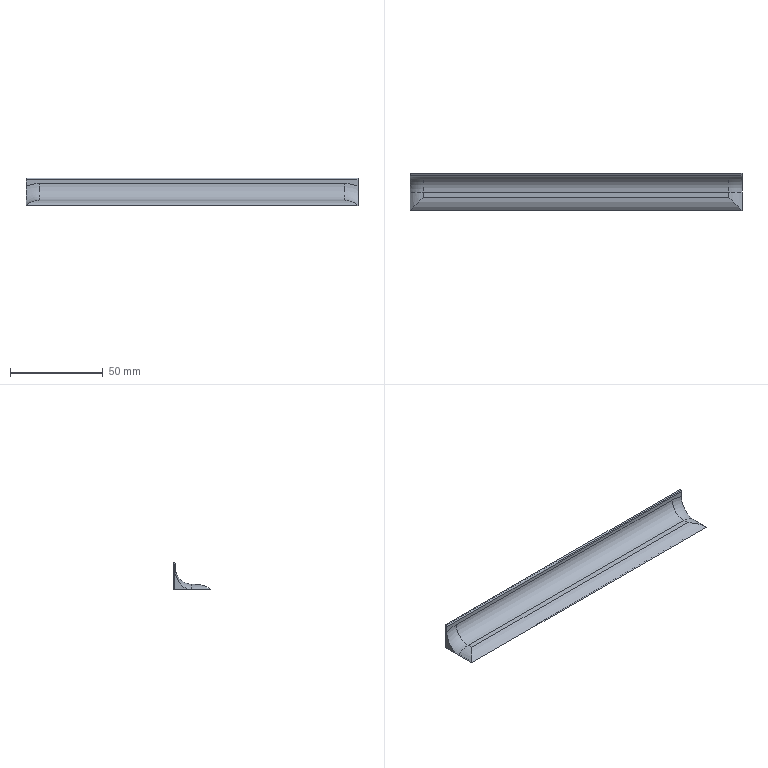Part | SolidWorks | features Fillet 3, ICE 2, Extrusion 1, Shell 1 | 1 solid | 23 faces | box 178.57 x 20 x 15 mm | volume 6954 mm3 | plane 12 | cylinder 9 | torus 2 | commonest cylinder face diameters 19 x4 20 x3 2 x1 18 x1
STEP:
#1=CARTESIAN_POINT('',(-88.785,9.5,0.));
#2=VERTEX_POINT('',#1);
#3=CARTESIAN_POINT('',(-88.785,10.,0.));
#4=VERTEX_POINT('',#3);
#5=CARTESIAN_POINT('',(-88.785,9.5,0.));
#6=DIRECTION('',(0.,1.,0.));
#7=VECTOR('',#6,1000.);
#8=LINE('',#5,#7);
#9=EDGE_CURVE('',#2,#4,#8,.T.);
#10=ORIENTED_EDGE('',*,*,#9,.F.);
#11=CARTESIAN_POINT('',(88.785,9.5,0.));
#12=VERTEX_POINT('',#11);
#13=CARTESIAN_POINT('',(-88.785,9.5,0.));
#14=DIRECTION('',(-1.,0.,0.));
#15=VECTOR('',#14,1000.);
#16=LINE('',#13,#15);
#17=EDGE_CURVE('',#12,#2,#16,.T.);
#18=ORIENTED_EDGE('',*,*,#17,.F.);
#19=CARTESIAN_POINT('',(88.785,10.,0.));
#20=VERTEX_POINT('',#19);
#21=CARTESIAN_POINT('',(88.785,9.5,0.));
#22=DIRECTION('',(0.,1.,0.));
#23=VECTOR('',#22,1000.);
#24=LINE('',#21,#23);
#25=EDGE_CURVE('',#12,#20,#24,.T.);
#26=ORIENTED_EDGE('',*,*,#25,.T.);
#27=CARTESIAN_POINT('',(89.285,10.,0.));
#28=VERTEX_POINT('',#27);
#29=CARTESIAN_POINT('',(-89.285,10.,0.));
#30=DIRECTION('',(-1.,0.,0.));
#31=VECTOR('',#30,1000.);
#32=LINE('',#29,#31);
#33=EDGE_CURVE('',#28,#20,#32,.T.);
#34=ORIENTED_EDGE('',*,*,#33,.F.);
#35=CARTESIAN_POINT('',(89.285,0.,0.));
#36=VERTEX_POINT('',#35);
#37=CARTESIAN_POINT('',(89.285,10.,0.));
#38=DIRECTION('',(0.,-1.,0.));
#39=VECTOR('',#38,1000.);
#40=LINE('',#37,#39);
#41=EDGE_CURVE('',#28,#36,#40,.T.);
#42=ORIENTED_EDGE('',*,*,#41,.T.);
#43=CARTESIAN_POINT('',(89.285,-10.,0.));
#44=VERTEX_POINT('',#43);
#45=CARTESIAN_POINT('',(89.285,-10.,0.));
#46=DIRECTION('',(0.,1.,0.));
#47=VECTOR('',#46,1000.);
#48=LINE('',#45,#47);
#49=EDGE_CURVE('',#44,#36,#48,.T.);
#50=ORIENTED_EDGE('',*,*,#49,.F.);
#51=CARTESIAN_POINT('',(-89.285,-10.,0.));
#52=VERTEX_POINT('',#51);
#53=CARTESIAN_POINT('',(-89.285,-10.,0.));
#54=DIRECTION('',(1.,0.,0.));
#55=VECTOR('',#54,1000.);
#56=LINE('',#53,#55);
#57=EDGE_CURVE('',#52,#44,#56,.T.);
#58=ORIENTED_EDGE('',*,*,#57,.F.);
#59=CARTESIAN_POINT('',(-89.285,0.,0.));
#60=VERTEX_POINT('',#59);
#61=CARTESIAN_POINT('',(-89.285,-10.,0.));
#62=DIRECTION('',(0.,-1.,0.));
#63=VECTOR('',#62,1000.);
#64=LINE('',#61,#63);
#65=EDGE_CURVE('',#60,#52,#64,.T.);
#66=ORIENTED_EDGE('',*,*,#65,.F.);
#67=CARTESIAN_POINT('',(-89.285,10.,0.));
#68=VERTEX_POINT('',#67);
#69=CARTESIAN_POINT('',(-89.285,-10.,0.));
#70=DIRECTION('',(0.,-1.,0.));
#71=VECTOR('',#70,1000.);
#72=LINE('',#69,#71);
#73=EDGE_CURVE('',#68,#60,#72,.T.);
#74=ORIENTED_EDGE('',*,*,#73,.F.);
#75=CARTESIAN_POINT('',(-89.285,10.,0.));
#76=DIRECTION('',(-1.,0.,0.));
#77=VECTOR('',#76,1000.);
#78=LINE('',#75,#77);
#79=EDGE_CURVE('',#4,#68,#78,.T.);
#80=ORIENTED_EDGE('',*,*,#79,.F.);
#81=EDGE_LOOP('',(#10,#18,#26,#34,#42,#50,#58,#66,#74,#80));
#82=FACE_OUTER_BOUND('',#81,.T.);
#83=CARTESIAN_POINT('',(88.566,-9.281,0.));
#84=VERTEX_POINT('',#83);
#85=CARTESIAN_POINT('',(88.566,9.,0.));
#86=VERTEX_POINT('',#85);
#87=CARTESIAN_POINT('',(88.566,-9.281,0.));
#88=DIRECTION('',(0.,1.,0.));
#89=VECTOR('',#88,1000.);
#90=LINE('',#87,#89);
#91=EDGE_CURVE('',#84,#86,#90,.T.);
#92=ORIENTED_EDGE('',*,*,#91,.T.);
#93=CARTESIAN_POINT('',(-88.566,9.,0.));
#94=VERTEX_POINT('',#93);
#95=CARTESIAN_POINT('',(89.285,9.,0.));
#96=DIRECTION('',(-1.,0.,0.));
#97=VECTOR('',#96,1000.);
#98=LINE('',#95,#97);
#99=EDGE_CURVE('',#86,#94,#98,.T.);
#100=ORIENTED_EDGE('',*,*,#99,.T.);
#101=CARTESIAN_POINT('',(-88.566,-9.281,0.));
#102=VERTEX_POINT('',#101);
#103=CARTESIAN_POINT('',(-88.566,9.281,0.));
#104=DIRECTION('',(0.,-1.,0.));
#105=VECTOR('',#104,1000.);
#106=LINE('',#103,#105);
#107=EDGE_CURVE('',#94,#102,#106,.T.);
#108=ORIENTED_EDGE('',*,*,#107,.T.);
#109=CARTESIAN_POINT('',(-88.566,-9.281,0.));
#110=DIRECTION('',(1.,0.,0.));
#111=VECTOR('',#110,1000.);
#112=LINE('',#109,#111);
#113=EDGE_CURVE('',#102,#84,#112,.T.);
#114=ORIENTED_EDGE('',*,*,#113,.T.);
#115=EDGE_LOOP('',(#92,#100,#108,#114));
#116=FACE_BOUND('',#115,.T.);
#117=CARTESIAN_POINT('',(0.,0.,0.));
#118=DIRECTION('',(0.,0.,-1.));
#119=DIRECTION('',(-1.,0.,0.));
#120=AXIS2_PLACEMENT_3D('',#117,#118,#119);
#121=PLANE('',#120);
#122=ADVANCED_FACE('',(#82,#116),#121,.T.);
#123=CARTESIAN_POINT('',(82.144,-2.859,3.));
#124=VERTEX_POINT('',#123);
#125=CARTESIAN_POINT('',(82.144,0.,3.));
#126=VERTEX_POINT('',#125);
#127=CARTESIAN_POINT('',(82.144,0.,3.));
#128=DIRECTION('',(0.,1.,0.));
#129=VECTOR('',#128,1000.);
#130=LINE('',#127,#129);
#131=EDGE_CURVE('',#124,#126,#130,.T.);
#132=ORIENTED_EDGE('',*,*,#131,.T.);
#133=CARTESIAN_POINT('',(-82.144,0.,3.));
#134=VERTEX_POINT('',#133);
#135=CARTESIAN_POINT('',(0.,0.,3.));
#136=DIRECTION('',(-1.,0.,0.));
#137=VECTOR('',#136,1000.);
#138=LINE('',#135,#137);
#139=EDGE_CURVE('',#126,#134,#138,.T.);
#140=ORIENTED_EDGE('',*,*,#139,.T.);
#141=CARTESIAN_POINT('',(-82.144,-2.859,3.));
#142=VERTEX_POINT('',#141);
#143=CARTESIAN_POINT('',(-82.144,0.,3.));
#144=DIRECTION('',(0.,-1.,0.));
#145=VECTOR('',#144,1000.);
#146=LINE('',#143,#145);
#147=EDGE_CURVE('',#134,#142,#146,.T.);
#148=ORIENTED_EDGE('',*,*,#147,.T.);
#149=CARTESIAN_POINT('',(0.,-2.859,3.));
#150=DIRECTION('',(1.,0.,0.));
#151=VECTOR('',#150,1000.);
#152=LINE('',#149,#151);
#153=EDGE_CURVE('',#142,#124,#152,.T.);
#154=ORIENTED_EDGE('',*,*,#153,.T.);
#155=EDGE_LOOP('',(#132,#140,#148,#154));
#156=FACE_OUTER_BOUND('',#155,.T.);
#157=CARTESIAN_POINT('',(0.,0.,3.));
#158=DIRECTION('',(0.,0.,-1.));
#159=DIRECTION('',(-1.,0.,0.));
#160=AXIS2_PLACEMENT_3D('',#157,#158,#159);
#161=PLANE('',#160);
#162=ADVANCED_FACE('',(#156),#161,.F.);
#163=ORIENTED_EDGE('',*,*,#147,.F.);
#164=CARTESIAN_POINT('',(-82.144,0.,-7.));
#165=DIRECTION('',(0.,-1.,0.));
#166=DIRECTION('',(0.,0.,-1.));
#167=AXIS2_PLACEMENT_3D('',#164,#165,#166);
#168=CIRCLE('',#167,10.);
#169=EDGE_CURVE('',#134,#60,#168,.T.);
#170=ORIENTED_EDGE('',*,*,#169,.T.);
#171=ORIENTED_EDGE('',*,*,#65,.T.);
#172=CARTESIAN_POINT('',(-82.144,-2.859,3.));
#173=CARTESIAN_POINT('',(-84.867,-5.582,3.));
#174=CARTESIAN_POINT('',(-87.378,-8.093,1.945));
#175=CARTESIAN_POINT('',(-89.285,-10.,0.));
#176=(BOUNDED_CURVE()B_SPLINE_CURVE(3,(#172,#173,#174,#175),.UNSPECIFIED.,.F.,.F.)B_SPLINE_CURVE_WITH_KNOTS((4,4),(1.571,2.366),.UNSPECIFIED.)CURVE()GEOMETRIC_REPRESENTATION_ITEM()RATIONAL_B_SPLINE_CURVE((1.,0.948,0.948,1.))REPRESENTATION_ITEM(''));
#177=EDGE_CURVE('',#142,#52,#176,.T.);
#178=ORIENTED_EDGE('',*,*,#177,.F.);
#179=EDGE_LOOP('',(#163,#170,#171,#178));
#180=FACE_OUTER_BOUND('',#179,.T.);
#181=CARTESIAN_POINT('',(-82.144,-10.,-7.));
#182=DIRECTION('',(0.,1.,0.));
#183=DIRECTION('',(0.,0.,1.));
#184=AXIS2_PLACEMENT_3D('',#181,#182,#183);
#185=CYLINDRICAL_SURFACE('',#184,10.);
#186=ADVANCED_FACE('',(#180),#185,.T.);
#187=ORIENTED_EDGE('',*,*,#49,.T.);
#188=CARTESIAN_POINT('',(82.144,0.,-7.));
#189=DIRECTION('',(0.,-1.,0.));
#190=DIRECTION('',(0.,0.,-1.));
#191=AXIS2_PLACEMENT_3D('',#188,#189,#190);
#192=CIRCLE('',#191,10.);
#193=EDGE_CURVE('',#36,#126,#192,.T.);
#194=ORIENTED_EDGE('',*,*,#193,.T.);
#195=ORIENTED_EDGE('',*,*,#131,.F.);
#196=CARTESIAN_POINT('',(89.285,-10.,0.));
#197=CARTESIAN_POINT('',(87.378,-8.093,1.945));
#198=CARTESIAN_POINT('',(84.867,-5.582,3.));
#199=CARTESIAN_POINT('',(82.144,-2.859,3.));
#200=(BOUNDED_CURVE()B_SPLINE_CURVE(3,(#196,#197,#198,#199),.UNSPECIFIED.,.F.,.F.)B_SPLINE_CURVE_WITH_KNOTS((4,4),(0.7754,1.571),.UNSPECIFIED.)CURVE()GEOMETRIC_REPRESENTATION_ITEM()RATIONAL_B_SPLINE_CURVE((1.,0.948,0.948,1.))REPRESENTATION_ITEM(''));
#201=EDGE_CURVE('',#44,#124,#200,.T.);
#202=ORIENTED_EDGE('',*,*,#201,.F.);
#203=EDGE_LOOP('',(#187,#194,#195,#202));
#204=FACE_OUTER_BOUND('',#203,.T.);
#205=CARTESIAN_POINT('',(82.144,-10.,-7.));
#206=DIRECTION('',(0.,-1.,0.));
#207=DIRECTION('',(0.,0.,-1.));
#208=AXIS2_PLACEMENT_3D('',#205,#206,#207);
#209=CYLINDRICAL_SURFACE('',#208,10.);
#210=ADVANCED_FACE('',(#204),#209,.T.);
#211=ORIENTED_EDGE('',*,*,#177,.T.);
#212=ORIENTED_EDGE('',*,*,#57,.T.);
#213=ORIENTED_EDGE('',*,*,#201,.T.);
#214=ORIENTED_EDGE('',*,*,#153,.F.);
#215=EDGE_LOOP('',(#211,#212,#213,#214));
#216=FACE_OUTER_BOUND('',#215,.T.);
#217=CARTESIAN_POINT('',(-89.285,-2.859,-7.));
#218=DIRECTION('',(-1.,0.,0.));
#219=DIRECTION('',(0.,0.,1.));
#220=AXIS2_PLACEMENT_3D('',#217,#218,#219);
#221=CYLINDRICAL_SURFACE('',#220,10.);
#222=ADVANCED_FACE('',(#216),#221,.T.);
#223=CARTESIAN_POINT('',(-82.144,2.859,2.5));
#224=VERTEX_POINT('',#223);
#225=CARTESIAN_POINT('',(-82.144,-2.859,2.5));
#226=VERTEX_POINT('',#225);
#227=CARTESIAN_POINT('',(-82.144,0.,2.5));
#228=DIRECTION('',(0.,-1.,0.));
#229=VECTOR('',#228,1000.);
#230=LINE('',#227,#229);
#231=EDGE_CURVE('',#224,#226,#230,.T.);
#232=ORIENTED_EDGE('',*,*,#231,.F.);
#233=CARTESIAN_POINT('',(82.144,2.859,2.5));
#234=VERTEX_POINT('',#233);
#235=CARTESIAN_POINT('',(0.,2.859,2.5));
#236=DIRECTION('',(-1.,0.,0.));
#237=VECTOR('',#236,1000.);
#238=LINE('',#235,#237);
#239=EDGE_CURVE('',#234,#224,#238,.T.);
#240=ORIENTED_EDGE('',*,*,#239,.F.);
#241=CARTESIAN_POINT('',(82.144,-2.859,2.5));
#242=VERTEX_POINT('',#241);
#243=CARTESIAN_POINT('',(82.144,0.,2.5));
#244=DIRECTION('',(0.,1.,0.));
#245=VECTOR('',#244,1000.);
#246=LINE('',#243,#245);
#247=EDGE_CURVE('',#242,#234,#246,.T.);
#248=ORIENTED_EDGE('',*,*,#247,.F.);
#249=CARTESIAN_POINT('',(0.,-2.859,2.5));
#250=DIRECTION('',(1.,0.,0.));
#251=VECTOR('',#250,1000.);
#252=LINE('',#249,#251);
#253=EDGE_CURVE('',#226,#242,#252,.T.);
#254=ORIENTED_EDGE('',*,*,#253,.F.);
#255=EDGE_LOOP('',(#232,#240,#248,#254));
#256=FACE_OUTER_BOUND('',#255,.T.);
#257=CARTESIAN_POINT('',(0.,0.,2.5));
#258=DIRECTION('',(0.,0.,-1.));
#259=DIRECTION('',(-1.,0.,0.));
#260=AXIS2_PLACEMENT_3D('',#257,#258,#259);
#261=PLANE('',#260);
#262=ADVANCED_FACE('',(#256),#261,.T.);
#263=CARTESIAN_POINT('',(-88.285,9.,0.248));
#264=VERTEX_POINT('',#263);
#265=CARTESIAN_POINT('',(-82.144,2.859,2.5));
#266=CARTESIAN_POINT('',(-84.417,5.132,2.5));
#267=CARTESIAN_POINT('',(-86.551,7.266,1.717));
#268=CARTESIAN_POINT('',(-88.285,9.,0.248));
#269=(BOUNDED_CURVE()B_SPLINE_CURVE(3,(#265,#266,#267,#268),.UNSPECIFIED.,.F.,.F.)B_SPLINE_CURVE_WITH_KNOTS((4,4),(4.712,5.415),.UNSPECIFIED.)CURVE()GEOMETRIC_REPRESENTATION_ITEM()RATIONAL_B_SPLINE_CURVE((1.,0.9592,0.9592,1.))REPRESENTATION_ITEM(''));
#270=EDGE_CURVE('',#224,#264,#269,.T.);
#271=ORIENTED_EDGE('',*,*,#270,.T.);
#272=CARTESIAN_POINT('',(88.285,9.,0.248));
#273=VERTEX_POINT('',#272);
#274=CARTESIAN_POINT('',(-89.285,9.,0.248));
#275=DIRECTION('',(1.,0.,0.));
#276=VECTOR('',#275,1000.);
#277=LINE('',#274,#276);
#278=EDGE_CURVE('',#264,#273,#277,.T.);
#279=ORIENTED_EDGE('',*,*,#278,.T.);
#280=CARTESIAN_POINT('',(88.285,9.,0.248));
#281=CARTESIAN_POINT('',(86.551,7.266,1.717));
#282=CARTESIAN_POINT('',(84.417,5.132,2.5));
#283=CARTESIAN_POINT('',(82.144,2.859,2.5));
#284=(BOUNDED_CURVE()B_SPLINE_CURVE(3,(#280,#281,#282,#283),.UNSPECIFIED.,.F.,.F.)B_SPLINE_CURVE_WITH_KNOTS((4,4),(4.009,4.712),.UNSPECIFIED.)CURVE()GEOMETRIC_REPRESENTATION_ITEM()RATIONAL_B_SPLINE_CURVE((1.,0.9592,0.9592,1.))REPRESENTATION_ITEM(''));
#285=EDGE_CURVE('',#273,#234,#284,.T.);
#286=ORIENTED_EDGE('',*,*,#285,.T.);
#287=ORIENTED_EDGE('',*,*,#239,.T.);
#288=EDGE_LOOP('',(#271,#279,#286,#287));
#289=FACE_OUTER_BOUND('',#288,.T.);
#290=CARTESIAN_POINT('',(-89.285,2.859,-7.));
#291=DIRECTION('',(1.,0.,0.));
#292=DIRECTION('',(0.,0.,-1.));
#293=AXIS2_PLACEMENT_3D('',#290,#291,#292);
#294=CYLINDRICAL_SURFACE('',#293,9.5);
#295=ADVANCED_FACE('',(#289),#294,.F.);
#296=ORIENTED_EDGE('',*,*,#107,.F.);
#297=CARTESIAN_POINT('',(-82.144,9.,-7.));
#298=DIRECTION('',(0.,1.,0.));
#299=DIRECTION('',(0.,0.,-1.));
#300=AXIS2_PLACEMENT_3D('',#297,#298,#299);
#301=CIRCLE('',#300,9.5);
#302=EDGE_CURVE('',#94,#264,#301,.T.);
#303=ORIENTED_EDGE('',*,*,#302,.T.);
#304=ORIENTED_EDGE('',*,*,#270,.F.);
#305=ORIENTED_EDGE('',*,*,#231,.T.);
#306=CARTESIAN_POINT('',(-82.144,-2.859,2.5));
#307=CARTESIAN_POINT('',(-84.55,-5.265,2.5));
#308=CARTESIAN_POINT('',(-86.793,-7.508,1.627));
#309=CARTESIAN_POINT('',(-88.566,-9.281,0.));
#310=(BOUNDED_CURVE()B_SPLINE_CURVE(3,(#306,#307,#308,#309),.UNSPECIFIED.,.F.,.F.)B_SPLINE_CURVE_WITH_KNOTS((4,4),(4.712,5.455),.UNSPECIFIED.)CURVE()GEOMETRIC_REPRESENTATION_ITEM()RATIONAL_B_SPLINE_CURVE((1.,0.9546,0.9546,1.))REPRESENTATION_ITEM(''));
#311=EDGE_CURVE('',#226,#102,#310,.T.);
#312=ORIENTED_EDGE('',*,*,#311,.T.);
#313=EDGE_LOOP('',(#296,#303,#304,#305,#312));
#314=FACE_OUTER_BOUND('',#313,.T.);
#315=CARTESIAN_POINT('',(-82.144,-10.,-7.));
#316=DIRECTION('',(0.,1.,0.));
#317=DIRECTION('',(0.,0.,1.));
#318=AXIS2_PLACEMENT_3D('',#315,#316,#317);
#319=CYLINDRICAL_SURFACE('',#318,9.5);
#320=ADVANCED_FACE('',(#314),#319,.F.);
#321=ORIENTED_EDGE('',*,*,#285,.F.);
#322=CARTESIAN_POINT('',(82.144,9.,-7.));
#323=DIRECTION('',(0.,1.,0.));
#324=DIRECTION('',(0.,0.,-1.));
#325=AXIS2_PLACEMENT_3D('',#322,#323,#324);
#326=CIRCLE('',#325,9.5);
#327=EDGE_CURVE('',#273,#86,#326,.T.);
#328=ORIENTED_EDGE('',*,*,#327,.T.);
#329=ORIENTED_EDGE('',*,*,#91,.F.);
#330=CARTESIAN_POINT('',(88.566,-9.281,0.));
#331=CARTESIAN_POINT('',(86.793,-7.508,1.627));
#332=CARTESIAN_POINT('',(84.55,-5.265,2.5));
#333=CARTESIAN_POINT('',(82.144,-2.859,2.5));
#334=(BOUNDED_CURVE()B_SPLINE_CURVE(3,(#330,#331,#332,#333),.UNSPECIFIED.,.F.,.F.)B_SPLINE_CURVE_WITH_KNOTS((4,4),(3.97,4.712),.UNSPECIFIED.)CURVE()GEOMETRIC_REPRESENTATION_ITEM()RATIONAL_B_SPLINE_CURVE((1.,0.9546,0.9546,1.))REPRESENTATION_ITEM(''));
#335=EDGE_CURVE('',#84,#242,#334,.T.);
#336=ORIENTED_EDGE('',*,*,#335,.T.);
#337=ORIENTED_EDGE('',*,*,#247,.T.);
#338=EDGE_LOOP('',(#321,#328,#329,#336,#337));
#339=FACE_OUTER_BOUND('',#338,.T.);
#340=CARTESIAN_POINT('',(82.144,-10.,-7.));
#341=DIRECTION('',(0.,-1.,0.));
#342=DIRECTION('',(0.,0.,-1.));
#343=AXIS2_PLACEMENT_3D('',#340,#341,#342);
#344=CYLINDRICAL_SURFACE('',#343,9.5);
#345=ADVANCED_FACE('',(#339),#344,.F.);
#346=ORIENTED_EDGE('',*,*,#311,.F.);
#347=ORIENTED_EDGE('',*,*,#253,.T.);
#348=ORIENTED_EDGE('',*,*,#335,.F.);
#349=ORIENTED_EDGE('',*,*,#113,.F.);
#350=EDGE_LOOP('',(#346,#347,#348,#349));
#351=FACE_OUTER_BOUND('',#350,.T.);
#352=CARTESIAN_POINT('',(-89.285,-2.859,-7.));
#353=DIRECTION('',(-1.,0.,0.));
#354=DIRECTION('',(0.,0.,1.));
#355=AXIS2_PLACEMENT_3D('',#352,#353,#354);
#356=CYLINDRICAL_SURFACE('',#355,9.5);
#357=ADVANCED_FACE('',(#351),#356,.F.);
#358=ORIENTED_EDGE('',*,*,#302,.F.);
#359=ORIENTED_EDGE('',*,*,#99,.F.);
#360=ORIENTED_EDGE('',*,*,#327,.F.);
#361=ORIENTED_EDGE('',*,*,#278,.F.);
#362=EDGE_LOOP('',(#358,#359,#360,#361));
#363=FACE_OUTER_BOUND('',#362,.T.);
#364=CARTESIAN_POINT('',(89.285,9.,15.));
#365=DIRECTION('',(0.,-1.,0.));
#366=DIRECTION('',(0.,0.,-1.));
#367=AXIS2_PLACEMENT_3D('',#364,#365,#366);
#368=PLANE('',#367);
#369=ADVANCED_FACE('',(#363),#368,.T.);
#370=CARTESIAN_POINT('',(89.285,10.,15.));
#371=VERTEX_POINT('',#370);
#372=CARTESIAN_POINT('',(89.285,10.,15.));
#373=DIRECTION('',(0.,0.,-1.));
#374=VECTOR('',#373,1000.);
#375=LINE('',#372,#374);
#376=EDGE_CURVE('',#371,#28,#375,.T.);
#377=ORIENTED_EDGE('',*,*,#376,.F.);
#378=CARTESIAN_POINT('',(89.285,9.,14.));
#379=VERTEX_POINT('',#378);
#380=CARTESIAN_POINT('',(89.285,10.,14.));
#381=DIRECTION('',(1.,0.,0.));
#382=DIRECTION('',(0.,0.,-1.));
#383=AXIS2_PLACEMENT_3D('',#380,#381,#382);
#384=CIRCLE('',#383,1.);
#385=EDGE_CURVE('',#371,#379,#384,.T.);
#386=ORIENTED_EDGE('',*,*,#385,.T.);
#387=CARTESIAN_POINT('',(89.285,9.,10.607));
#388=VERTEX_POINT('',#387);
#389=CARTESIAN_POINT('',(89.285,9.,15.));
#390=DIRECTION('',(0.,0.,-1.));
#391=VECTOR('',#390,1000.);
#392=LINE('',#389,#391);
#393=EDGE_CURVE('',#379,#388,#392,.T.);
#394=ORIENTED_EDGE('',*,*,#393,.T.);
#395=CARTESIAN_POINT('',(89.285,9.,10.607));
#396=CARTESIAN_POINT('',(89.285,9.,9.965));
#397=CARTESIAN_POINT('',(89.285,8.942,9.334));
#398=CARTESIAN_POINT('',(89.285,8.718,8.09));
#399=CARTESIAN_POINT('',(89.285,8.553,7.476));
#400=CARTESIAN_POINT('',(89.285,8.117,6.272));
#401=CARTESIAN_POINT('',(89.285,7.851,5.696));
#402=CARTESIAN_POINT('',(89.285,7.387,4.868));
#403=CARTESIAN_POINT('',(89.285,7.221,4.599));
#404=CARTESIAN_POINT('',(89.285,6.866,4.072));
#405=CARTESIAN_POINT('',(89.285,6.676,3.813));
#406=CARTESIAN_POINT('',(89.285,6.078,3.064));
#407=CARTESIAN_POINT('',(89.285,5.644,2.604));
#408=CARTESIAN_POINT('',(89.285,4.701,1.766));
#409=CARTESIAN_POINT('',(89.285,4.193,1.387));
#410=CARTESIAN_POINT('',(89.285,3.087,0.7335));
#411=CARTESIAN_POINT('',(89.285,2.508,0.4703));
#412=CARTESIAN_POINT('',(89.285,1.591,0.1935));
#413=CARTESIAN_POINT('',(89.285,1.275,0.1212));
#414=CARTESIAN_POINT('',(89.285,0.6417,0.02471));
#415=CARTESIAN_POINT('',(89.285,0.3223,0.));
#416=CARTESIAN_POINT('',(89.285,0.,0.));
#417=B_SPLINE_CURVE_WITH_KNOTS('',3,(#395,#396,#397,#398,#399,#400,#401,#402,#403,#404,#405,#406,#407,#408,#409,#410,#411,#412,#413,#414,#415,#416),.UNSPECIFIED.,.F.,.F.,(4,2,2,2,2,2,2,2,2,2,4),(0.,0.001896,0.003792,0.005687,0.006635,0.007583,0.009479,0.01137,0.01327,0.01422,0.01517),.UNSPECIFIED.);
#418=EDGE_CURVE('',#388,#36,#417,.T.);
#419=ORIENTED_EDGE('',*,*,#418,.T.);
#420=ORIENTED_EDGE('',*,*,#41,.F.);
#421=EDGE_LOOP('',(#377,#386,#394,#419,#420));
#422=FACE_OUTER_BOUND('',#421,.T.);
#423=CARTESIAN_POINT('',(89.285,10.,15.));
#424=DIRECTION('',(1.,0.,0.));
#425=DIRECTION('',(0.,0.,-1.));
#426=AXIS2_PLACEMENT_3D('',#423,#424,#425);
#427=PLANE('',#426);
#428=ADVANCED_FACE('',(#422),#427,.T.);
#429=CARTESIAN_POINT('',(-88.785,10.,14.5));
#430=VERTEX_POINT('',#429);
#431=CARTESIAN_POINT('',(-88.785,10.,0.));
#432=DIRECTION('',(0.,0.,1.));
#433=VECTOR('',#432,1000.);
#434=LINE('',#431,#433);
#435=EDGE_CURVE('',#4,#430,#434,.T.);
#436=ORIENTED_EDGE('',*,*,#435,.F.);
#437=ORIENTED_EDGE('',*,*,#79,.T.);
#438=CARTESIAN_POINT('',(-89.285,10.,15.));
#439=VERTEX_POINT('',#438);
#440=CARTESIAN_POINT('',(-89.285,10.,15.));
#441=DIRECTION('',(0.,0.,-1.));
#442=VECTOR('',#441,1000.);
#443=LINE('',#440,#442);
#444=EDGE_CURVE('',#439,#68,#443,.T.);
#445=ORIENTED_EDGE('',*,*,#444,.F.);
#446=CARTESIAN_POINT('',(89.285,10.,15.));
#447=DIRECTION('',(1.,0.,0.));
#448=VECTOR('',#447,1000.);
#449=LINE('',#446,#448);
#450=EDGE_CURVE('',#439,#371,#449,.T.);
#451=ORIENTED_EDGE('',*,*,#450,.T.);
#452=ORIENTED_EDGE('',*,*,#376,.T.);
#453=ORIENTED_EDGE('',*,*,#33,.T.);
#454=CARTESIAN_POINT('',(88.785,10.,14.5));
#455=VERTEX_POINT('',#454);
#456=CARTESIAN_POINT('',(88.785,10.,0.));
#457=DIRECTION('',(0.,0.,-1.));
#458=VECTOR('',#457,1000.);
#459=LINE('',#456,#458);
#460=EDGE_CURVE('',#455,#20,#459,.T.);
#461=ORIENTED_EDGE('',*,*,#460,.F.);
#462=CARTESIAN_POINT('',(-88.785,10.,14.5));
#463=DIRECTION('',(1.,0.,0.));
#464=VECTOR('',#463,1000.);
#465=LINE('',#462,#464);
#466=EDGE_CURVE('',#430,#455,#465,.T.);
#467=ORIENTED_EDGE('',*,*,#466,.F.);
#468=EDGE_LOOP('',(#436,#437,#445,#451,#452,#453,#461,#467));
#469=FACE_OUTER_BOUND('',#468,.T.);
#470=CARTESIAN_POINT('',(89.285,10.,15.));
#471=DIRECTION('',(0.,1.,0.));
#472=DIRECTION('',(0.,0.,1.));
#473=AXIS2_PLACEMENT_3D('',#470,#471,#472);
#474=PLANE('',#473);
#475=ADVANCED_FACE('',(#469),#474,.T.);
#476=CARTESIAN_POINT('',(-89.285,9.,14.));
#477=VERTEX_POINT('',#476);
#478=CARTESIAN_POINT('',(-89.285,9.,10.607));
#479=VERTEX_POINT('',#478);
#480=CARTESIAN_POINT('',(-89.285,9.,15.));
#481=DIRECTION('',(0.,0.,-1.));
#482=VECTOR('',#481,1000.);
#483=LINE('',#480,#482);
#484=EDGE_CURVE('',#477,#479,#483,.T.);
#485=ORIENTED_EDGE('',*,*,#484,.F.);
#486=CARTESIAN_POINT('',(-89.285,10.,14.));
#487=DIRECTION('',(-1.,0.,0.));
#488=DIRECTION('',(0.,0.,1.));
#489=AXIS2_PLACEMENT_3D('',#486,#487,#488);
#490=CIRCLE('',#489,1.);
#491=EDGE_CURVE('',#477,#439,#490,.T.);
#492=ORIENTED_EDGE('',*,*,#491,.T.);
#493=ORIENTED_EDGE('',*,*,#444,.T.);
#494=ORIENTED_EDGE('',*,*,#73,.T.);
#495=CARTESIAN_POINT('',(-89.285,0.,0.));
#496=CARTESIAN_POINT('',(-89.285,0.6442,0.));
#497=CARTESIAN_POINT('',(-89.285,1.269,0.09828));
#498=CARTESIAN_POINT('',(-89.285,2.181,0.3709));
#499=CARTESIAN_POINT('',(-89.285,2.483,0.4837));
#500=CARTESIAN_POINT('',(-89.285,3.068,0.7434));
#501=CARTESIAN_POINT('',(-89.285,3.35,0.8899));
#502=CARTESIAN_POINT('',(-89.285,3.898,1.212));
#503=CARTESIAN_POINT('',(-89.285,4.163,1.388));
#504=CARTESIAN_POINT('',(-89.285,4.679,1.766));
#505=CARTESIAN_POINT('',(-89.285,4.928,1.968));
#506=CARTESIAN_POINT('',(-89.285,5.641,2.601));
#507=CARTESIAN_POINT('',(-89.285,6.075,3.061));
#508=CARTESIAN_POINT('',(-89.285,6.669,3.803));
#509=CARTESIAN_POINT('',(-89.285,6.857,4.059));
#510=CARTESIAN_POINT('',(-89.285,7.214,4.588));
#511=CARTESIAN_POINT('',(-89.285,7.382,4.861));
#512=CARTESIAN_POINT('',(-89.285,7.849,5.692));
#513=CARTESIAN_POINT('',(-89.285,8.114,6.266));
#514=CARTESIAN_POINT('',(-89.285,8.547,7.457));
#515=CARTESIAN_POINT('',(-89.285,8.716,8.078));
#516=CARTESIAN_POINT('',(-89.285,8.942,9.332));
#517=CARTESIAN_POINT('',(-89.285,9.,9.966));
#518=CARTESIAN_POINT('',(-89.285,9.,10.607));
#519=B_SPLINE_CURVE_WITH_KNOTS('',3,(#495,#496,#497,#498,#499,#500,#501,#502,#503,#504,#505,#506,#507,#508,#509,#510,#511,#512,#513,#514,#515,#516,#517,#518),.UNSPECIFIED.,.F.,.F.,(4,2,2,2,2,2,2,2,2,2,2,4),(0.,0.001896,0.002844,0.003792,0.00474,0.005688,0.007584,0.008532,0.00948,0.01138,0.01327,0.01517),.UNSPECIFIED.);
#520=EDGE_CURVE('',#60,#479,#519,.T.);
#521=ORIENTED_EDGE('',*,*,#520,.T.);
#522=EDGE_LOOP('',(#485,#492,#493,#494,#521));
#523=FACE_OUTER_BOUND('',#522,.T.);
#524=CARTESIAN_POINT('',(-89.285,10.,15.));
#525=DIRECTION('',(-1.,0.,0.));
#526=DIRECTION('',(0.,0.,1.));
#527=AXIS2_PLACEMENT_3D('',#524,#525,#526);
#528=PLANE('',#527);
#529=ADVANCED_FACE('',(#523),#528,.T.);
#530=ORIENTED_EDGE('',*,*,#393,.F.);
#531=CARTESIAN_POINT('',(-89.285,9.,14.));
#532=DIRECTION('',(-1.,0.,0.));
#533=VECTOR('',#532,1000.);
#534=LINE('',#531,#533);
#535=EDGE_CURVE('',#379,#477,#534,.T.);
#536=ORIENTED_EDGE('',*,*,#535,.T.);
#537=ORIENTED_EDGE('',*,*,#484,.T.);
#538=CARTESIAN_POINT('',(-82.144,9.,12.));
#539=VERTEX_POINT('',#538);
#540=CARTESIAN_POINT('',(-82.144,9.,-7.));
#541=DIRECTION('',(0.,1.,0.));
#542=DIRECTION('',(0.,0.,-1.));
#543=AXIS2_PLACEMENT_3D('',#540,#541,#542);
#544=CIRCLE('',#543,19.);
#545=EDGE_CURVE('',#479,#539,#544,.T.);
#546=ORIENTED_EDGE('',*,*,#545,.T.);
#547=CARTESIAN_POINT('',(82.144,9.,12.));
#548=VERTEX_POINT('',#547);
#549=CARTESIAN_POINT('',(89.285,9.,12.));
#550=DIRECTION('',(1.,0.,0.));
#551=VECTOR('',#550,1000.);
#552=LINE('',#549,#551);
#553=EDGE_CURVE('',#539,#548,#552,.T.);
#554=ORIENTED_EDGE('',*,*,#553,.T.);
#555=CARTESIAN_POINT('',(82.144,9.,-7.));
#556=DIRECTION('',(0.,1.,0.));
#557=DIRECTION('',(0.,0.,-1.));
#558=AXIS2_PLACEMENT_3D('',#555,#556,#557);
#559=CIRCLE('',#558,19.);
#560=EDGE_CURVE('',#548,#388,#559,.T.);
#561=ORIENTED_EDGE('',*,*,#560,.T.);
#562=EDGE_LOOP('',(#530,#536,#537,#546,#554,#561));
#563=FACE_OUTER_BOUND('',#562,.T.);
#564=CARTESIAN_POINT('',(89.285,9.,15.));
#565=DIRECTION('',(0.,-1.,0.));
#566=DIRECTION('',(0.,0.,-1.));
#567=AXIS2_PLACEMENT_3D('',#564,#565,#566);
#568=PLANE('',#567);
#569=ADVANCED_FACE('',(#563),#568,.T.);
#570=ORIENTED_EDGE('',*,*,#520,.F.);
#571=ORIENTED_EDGE('',*,*,#169,.F.);
#572=CARTESIAN_POINT('',(-82.144,0.,12.));
#573=DIRECTION('',(-1.,0.,0.));
#574=DIRECTION('',(0.,0.,-1.));
#575=AXIS2_PLACEMENT_3D('',#572,#573,#574);
#576=CIRCLE('',#575,9.);
#577=EDGE_CURVE('',#539,#134,#576,.T.);
#578=ORIENTED_EDGE('',*,*,#577,.F.);
#579=ORIENTED_EDGE('',*,*,#545,.F.);
#580=EDGE_LOOP('',(#570,#571,#578,#579));
#581=FACE_OUTER_BOUND('',#580,.T.);
#582=CARTESIAN_POINT('',(-82.144,0.,-7.));
#583=DIRECTION('',(0.,-1.,0.));
#584=DIRECTION('',(0.,0.,-1.));
#585=AXIS2_PLACEMENT_3D('',#582,#583,#584);
#586=TOROIDAL_SURFACE('',#585,19.,9.);
#587=ADVANCED_FACE('',(#581),#586,.F.);
#588=ORIENTED_EDGE('',*,*,#577,.T.);
#589=ORIENTED_EDGE('',*,*,#139,.F.);
#590=CARTESIAN_POINT('',(82.144,0.,12.));
#591=DIRECTION('',(-1.,0.,0.));
#592=DIRECTION('',(0.,0.,-1.));
#593=AXIS2_PLACEMENT_3D('',#590,#591,#592);
#594=CIRCLE('',#593,9.);
#595=EDGE_CURVE('',#548,#126,#594,.T.);
#596=ORIENTED_EDGE('',*,*,#595,.F.);
#597=ORIENTED_EDGE('',*,*,#553,.F.);
#598=EDGE_LOOP('',(#588,#589,#596,#597));
#599=FACE_OUTER_BOUND('',#598,.T.);
#600=CARTESIAN_POINT('',(89.285,0.,12.));
#601=DIRECTION('',(1.,0.,0.));
#602=DIRECTION('',(0.,0.,-1.));
#603=AXIS2_PLACEMENT_3D('',#600,#601,#602);
#604=CYLINDRICAL_SURFACE('',#603,9.);
#605=ADVANCED_FACE('',(#599),#604,.F.);
#606=ORIENTED_EDGE('',*,*,#595,.T.);
#607=ORIENTED_EDGE('',*,*,#193,.F.);
#608=ORIENTED_EDGE('',*,*,#418,.F.);
#609=ORIENTED_EDGE('',*,*,#560,.F.);
#610=EDGE_LOOP('',(#606,#607,#608,#609));
#611=FACE_OUTER_BOUND('',#610,.T.);
#612=CARTESIAN_POINT('',(82.144,0.,-7.));
#613=DIRECTION('',(0.,-1.,0.));
#614=DIRECTION('',(0.,0.,-1.));
#615=AXIS2_PLACEMENT_3D('',#612,#613,#614);
#616=TOROIDAL_SURFACE('',#615,19.,9.);
#617=ADVANCED_FACE('',(#611),#616,.F.);
#618=ORIENTED_EDGE('',*,*,#385,.F.);
#619=ORIENTED_EDGE('',*,*,#450,.F.);
#620=ORIENTED_EDGE('',*,*,#491,.F.);
#621=ORIENTED_EDGE('',*,*,#535,.F.);
#622=EDGE_LOOP('',(#618,#619,#620,#621));
#623=FACE_OUTER_BOUND('',#622,.T.);
#624=CARTESIAN_POINT('',(89.285,10.,14.));
#625=DIRECTION('',(1.,0.,0.));
#626=DIRECTION('',(0.,0.,-1.));
#627=AXIS2_PLACEMENT_3D('',#624,#625,#626);
#628=CYLINDRICAL_SURFACE('',#627,1.);
#629=ADVANCED_FACE('',(#623),#628,.T.);
#630=ORIENTED_EDGE('',*,*,#435,.T.);
#631=CARTESIAN_POINT('',(-88.785,9.5,14.5));
#632=VERTEX_POINT('',#631);
#633=CARTESIAN_POINT('',(-88.785,9.5,14.5));
#634=DIRECTION('',(0.,1.,0.));
#635=VECTOR('',#634,1000.);
#636=LINE('',#633,#635);
#637=EDGE_CURVE('',#632,#430,#636,.T.);
#638=ORIENTED_EDGE('',*,*,#637,.F.);
#639=CARTESIAN_POINT('',(-88.785,9.5,0.));
#640=DIRECTION('',(0.,0.,1.));
#641=VECTOR('',#640,1000.);
#642=LINE('',#639,#641);
#643=EDGE_CURVE('',#2,#632,#642,.T.);
#644=ORIENTED_EDGE('',*,*,#643,.F.);
#645=ORIENTED_EDGE('',*,*,#9,.T.);
#646=EDGE_LOOP('',(#630,#638,#644,#645));
#647=FACE_OUTER_BOUND('',#646,.T.);
#648=CARTESIAN_POINT('',(-88.785,9.5,0.));
#649=DIRECTION('',(-1.,0.,0.));
#650=DIRECTION('',(0.,0.,1.));
#651=AXIS2_PLACEMENT_3D('',#648,#649,#650);
#652=PLANE('',#651);
#653=ADVANCED_FACE('',(#647),#652,.F.);
#654=ORIENTED_EDGE('',*,*,#460,.T.);
#655=ORIENTED_EDGE('',*,*,#25,.F.);
#656=CARTESIAN_POINT('',(88.785,9.5,14.5));
#657=VERTEX_POINT('',#656);
#658=CARTESIAN_POINT('',(88.785,9.5,0.));
#659=DIRECTION('',(0.,0.,-1.));
#660=VECTOR('',#659,1000.);
#661=LINE('',#658,#660);
#662=EDGE_CURVE('',#657,#12,#661,.T.);
#663=ORIENTED_EDGE('',*,*,#662,.F.);
#664=CARTESIAN_POINT('',(88.785,9.5,14.5));
#665=DIRECTION('',(0.,1.,0.));
#666=VECTOR('',#665,1000.);
#667=LINE('',#664,#666);
#668=EDGE_CURVE('',#657,#455,#667,.T.);
#669=ORIENTED_EDGE('',*,*,#668,.T.);
#670=EDGE_LOOP('',(#654,#655,#663,#669));
#671=FACE_OUTER_BOUND('',#670,.T.);
#672=CARTESIAN_POINT('',(88.785,9.5,0.));
#673=DIRECTION('',(1.,0.,0.));
#674=DIRECTION('',(0.,0.,-1.));
#675=AXIS2_PLACEMENT_3D('',#672,#673,#674);
#676=PLANE('',#675);
#677=ADVANCED_FACE('',(#671),#676,.F.);
#678=ORIENTED_EDGE('',*,*,#466,.T.);
#679=ORIENTED_EDGE('',*,*,#668,.F.);
#680=CARTESIAN_POINT('',(-88.785,9.5,14.5));
#681=DIRECTION('',(1.,0.,0.));
#682=VECTOR('',#681,1000.);
#683=LINE('',#680,#682);
#684=EDGE_CURVE('',#632,#657,#683,.T.);
#685=ORIENTED_EDGE('',*,*,#684,.F.);
#686=ORIENTED_EDGE('',*,*,#637,.T.);
#687=EDGE_LOOP('',(#678,#679,#685,#686));
#688=FACE_OUTER_BOUND('',#687,.T.);
#689=CARTESIAN_POINT('',(-88.785,9.5,14.5));
#690=DIRECTION('',(0.,0.,1.));
#691=DIRECTION('',(1.,0.,0.));
#692=AXIS2_PLACEMENT_3D('',#689,#690,#691);
#693=PLANE('',#692);
#694=ADVANCED_FACE('',(#688),#693,.F.);
#695=ORIENTED_EDGE('',*,*,#643,.T.);
#696=ORIENTED_EDGE('',*,*,#684,.T.);
#697=ORIENTED_EDGE('',*,*,#662,.T.);
#698=ORIENTED_EDGE('',*,*,#17,.T.);
#699=EDGE_LOOP('',(#695,#696,#697,#698));
#700=FACE_OUTER_BOUND('',#699,.T.);
#701=CARTESIAN_POINT('',(0.,9.5,0.));
#702=DIRECTION('',(0.,1.,0.));
#703=DIRECTION('',(0.,0.,1.));
#704=AXIS2_PLACEMENT_3D('',#701,#702,#703);
#705=PLANE('',#704);
#706=ADVANCED_FACE('',(#700),#705,.T.);
#707=CLOSED_SHELL('',(#122,#162,#186,#210,#222,#262,#295,#320,#345,#357,#369,#428,#475,#529,#569,#587,#605,#617,#629,#653,#677,#694,#706));
#708=MANIFOLD_SOLID_BREP('',#707);
#709=CARTESIAN_POINT('',(0.,0.,0.));
#710=DIRECTION('',(0.,0.,1.));
#711=DIRECTION('',(1.,0.,0.));
#712=AXIS2_PLACEMENT_3D('',#709,#710,#711);
#713=(LENGTH_UNIT()NAMED_UNIT(*)SI_UNIT(.MILLI.,.METRE.));
#714=UNCERTAINTY_MEASURE_WITH_UNIT(LENGTH_MEASURE(0.00001),#713,'','');
#715=(NAMED_UNIT(*)PLANE_ANGLE_UNIT()SI_UNIT($,.RADIAN.));
#716=(NAMED_UNIT(*)SI_UNIT($,.STERADIAN.)SOLID_ANGLE_UNIT());
#717=(GEOMETRIC_REPRESENTATION_CONTEXT(3)GLOBAL_UNCERTAINTY_ASSIGNED_CONTEXT((#714))GLOBAL_UNIT_ASSIGNED_CONTEXT((#713,#715,#716))REPRESENTATION_CONTEXT('',''));
#718=ADVANCED_BREP_SHAPE_REPRESENTATION('',(#708,#712),#717);